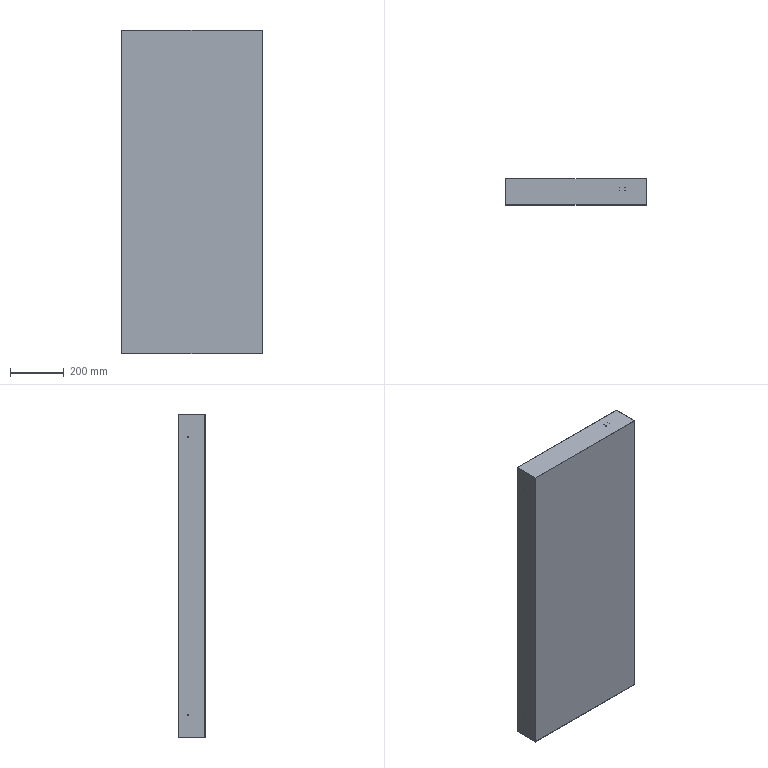Part | SolidWorks | features BaseBody 1 | 1 solid | 27 faces | box 521.763 x 96.993 x 1200 mm | volume 956249 mm3 | cylinder 16 | plane 11 | commonest cylinder face diameters 1.828 x8 3 x8
STEP:
#1=CARTESIAN_POINT('',(-260.881,-535.859,518.28));
#2=VERTEX_POINT('',#1);
#3=CARTESIAN_POINT('',(-260.881,-535.859,515.28));
#4=VERTEX_POINT('',#3);
#5=CARTESIAN_POINT('',(-260.881,-535.859,516.78));
#6=DIRECTION('',(1.,0.,0.));
#7=DIRECTION('',(0.,0.,-1.));
#8=AXIS2_PLACEMENT_3D('',#5,#6,#7);
#9=CIRCLE('',#8,1.5);
#10=EDGE_CURVE('',#2,#4,#9,.T.);
#11=ORIENTED_EDGE('',*,*,#10,.F.);
#12=CARTESIAN_POINT('',(-259.881,-535.859,518.28));
#13=VERTEX_POINT('',#12);
#14=CARTESIAN_POINT('',(-260.881,-535.859,518.28));
#15=DIRECTION('',(1.,0.,0.));
#16=VECTOR('',#15,1000.);
#17=LINE('',#14,#16);
#18=EDGE_CURVE('',#2,#13,#17,.T.);
#19=ORIENTED_EDGE('',*,*,#18,.T.);
#20=CARTESIAN_POINT('',(-259.881,-535.859,515.28));
#21=VERTEX_POINT('',#20);
#22=CARTESIAN_POINT('',(-259.881,-535.859,516.78));
#23=DIRECTION('',(-1.,0.,0.));
#24=DIRECTION('',(0.,0.,-1.));
#25=AXIS2_PLACEMENT_3D('',#22,#23,#24);
#26=CIRCLE('',#25,1.5);
#27=EDGE_CURVE('',#21,#13,#26,.T.);
#28=ORIENTED_EDGE('',*,*,#27,.F.);
#29=CARTESIAN_POINT('',(-260.881,-535.859,515.28));
#30=DIRECTION('',(1.,0.,0.));
#31=VECTOR('',#30,1000.);
#32=LINE('',#29,#31);
#33=EDGE_CURVE('',#4,#21,#32,.T.);
#34=ORIENTED_EDGE('',*,*,#33,.F.);
#35=EDGE_LOOP('',(#11,#19,#28,#34));
#36=FACE_OUTER_BOUND('',#35,.T.);
#37=CARTESIAN_POINT('',(-260.881,-535.859,516.78));
#38=DIRECTION('',(1.,0.,0.));
#39=DIRECTION('',(0.,0.,-1.));
#40=AXIS2_PLACEMENT_3D('',#37,#38,#39);
#41=CYLINDRICAL_SURFACE('',#40,1.5);
#42=ADVANCED_FACE('',(#36),#41,.F.);
#43=CARTESIAN_POINT('',(-260.881,-535.859,-515.72));
#44=VERTEX_POINT('',#43);
#45=CARTESIAN_POINT('',(-260.881,-535.859,-518.72));
#46=VERTEX_POINT('',#45);
#47=CARTESIAN_POINT('',(-260.881,-535.859,-517.22));
#48=DIRECTION('',(1.,0.,0.));
#49=DIRECTION('',(0.,0.,-1.));
#50=AXIS2_PLACEMENT_3D('',#47,#48,#49);
#51=CIRCLE('',#50,1.5);
#52=EDGE_CURVE('',#44,#46,#51,.T.);
#53=ORIENTED_EDGE('',*,*,#52,.F.);
#54=CARTESIAN_POINT('',(-259.881,-535.859,-515.72));
#55=VERTEX_POINT('',#54);
#56=CARTESIAN_POINT('',(-260.881,-535.859,-515.72));
#57=DIRECTION('',(1.,0.,0.));
#58=VECTOR('',#57,1000.);
#59=LINE('',#56,#58);
#60=EDGE_CURVE('',#44,#55,#59,.T.);
#61=ORIENTED_EDGE('',*,*,#60,.T.);
#62=CARTESIAN_POINT('',(-259.881,-535.859,-518.72));
#63=VERTEX_POINT('',#62);
#64=CARTESIAN_POINT('',(-259.881,-535.859,-517.22));
#65=DIRECTION('',(-1.,0.,0.));
#66=DIRECTION('',(0.,0.,-1.));
#67=AXIS2_PLACEMENT_3D('',#64,#65,#66);
#68=CIRCLE('',#67,1.5);
#69=EDGE_CURVE('',#63,#55,#68,.T.);
#70=ORIENTED_EDGE('',*,*,#69,.F.);
#71=CARTESIAN_POINT('',(-260.881,-535.859,-518.72));
#72=DIRECTION('',(1.,0.,0.));
#73=VECTOR('',#72,1000.);
#74=LINE('',#71,#73);
#75=EDGE_CURVE('',#46,#63,#74,.T.);
#76=ORIENTED_EDGE('',*,*,#75,.F.);
#77=EDGE_LOOP('',(#53,#61,#70,#76));
#78=FACE_OUTER_BOUND('',#77,.T.);
#79=CARTESIAN_POINT('',(-260.881,-535.859,-517.22));
#80=DIRECTION('',(1.,0.,0.));
#81=DIRECTION('',(0.,0.,-1.));
#82=AXIS2_PLACEMENT_3D('',#79,#80,#81);
#83=CYLINDRICAL_SURFACE('',#82,1.5);
#84=ADVANCED_FACE('',(#78),#83,.F.);
#85=CARTESIAN_POINT('',(182.261,-534.957,600.));
#86=VERTEX_POINT('',#85);
#87=CARTESIAN_POINT('',(180.433,-534.957,600.));
#88=VERTEX_POINT('',#87);
#89=CARTESIAN_POINT('',(181.347,-534.957,600.));
#90=DIRECTION('',(0.,0.,-1.));
#91=DIRECTION('',(-1.,0.,0.));
#92=AXIS2_PLACEMENT_3D('',#89,#90,#91);
#93=CIRCLE('',#92,0.9139);
#94=EDGE_CURVE('',#86,#88,#93,.T.);
#95=ORIENTED_EDGE('',*,*,#94,.F.);
#96=CARTESIAN_POINT('',(182.261,-534.957,599.));
#97=VERTEX_POINT('',#96);
#98=CARTESIAN_POINT('',(182.261,-534.957,600.));
#99=DIRECTION('',(0.,0.,-1.));
#100=VECTOR('',#99,1000.);
#101=LINE('',#98,#100);
#102=EDGE_CURVE('',#86,#97,#101,.T.);
#103=ORIENTED_EDGE('',*,*,#102,.T.);
#104=CARTESIAN_POINT('',(180.433,-534.957,599.));
#105=VERTEX_POINT('',#104);
#106=CARTESIAN_POINT('',(181.347,-534.957,599.));
#107=DIRECTION('',(0.,0.,1.));
#108=DIRECTION('',(-1.,0.,0.));
#109=AXIS2_PLACEMENT_3D('',#106,#107,#108);
#110=CIRCLE('',#109,0.9139);
#111=EDGE_CURVE('',#105,#97,#110,.T.);
#112=ORIENTED_EDGE('',*,*,#111,.F.);
#113=CARTESIAN_POINT('',(180.433,-534.957,600.));
#114=DIRECTION('',(0.,0.,-1.));
#115=VECTOR('',#114,1000.);
#116=LINE('',#113,#115);
#117=EDGE_CURVE('',#88,#105,#116,.T.);
#118=ORIENTED_EDGE('',*,*,#117,.F.);
#119=EDGE_LOOP('',(#95,#103,#112,#118));
#120=FACE_OUTER_BOUND('',#119,.T.);
#121=CARTESIAN_POINT('',(181.347,-534.957,600.));
#122=DIRECTION('',(0.,0.,-1.));
#123=DIRECTION('',(-1.,0.,0.));
#124=AXIS2_PLACEMENT_3D('',#121,#122,#123);
#125=CYLINDRICAL_SURFACE('',#124,0.9139);
#126=ADVANCED_FACE('',(#120),#125,.F.);
#127=CARTESIAN_POINT('',(162.572,-534.957,600.));
#128=VERTEX_POINT('',#127);
#129=CARTESIAN_POINT('',(160.745,-534.957,600.));
#130=VERTEX_POINT('',#129);
#131=CARTESIAN_POINT('',(161.659,-534.957,600.));
#132=DIRECTION('',(0.,0.,-1.));
#133=DIRECTION('',(-1.,0.,0.));
#134=AXIS2_PLACEMENT_3D('',#131,#132,#133);
#135=CIRCLE('',#134,0.9139);
#136=EDGE_CURVE('',#128,#130,#135,.T.);
#137=ORIENTED_EDGE('',*,*,#136,.F.);
#138=CARTESIAN_POINT('',(162.572,-534.957,599.));
#139=VERTEX_POINT('',#138);
#140=CARTESIAN_POINT('',(162.572,-534.957,600.));
#141=DIRECTION('',(0.,0.,-1.));
#142=VECTOR('',#141,1000.);
#143=LINE('',#140,#142);
#144=EDGE_CURVE('',#128,#139,#143,.T.);
#145=ORIENTED_EDGE('',*,*,#144,.T.);
#146=CARTESIAN_POINT('',(160.745,-534.957,599.));
#147=VERTEX_POINT('',#146);
#148=CARTESIAN_POINT('',(161.659,-534.957,599.));
#149=DIRECTION('',(0.,0.,1.));
#150=DIRECTION('',(-1.,0.,0.));
#151=AXIS2_PLACEMENT_3D('',#148,#149,#150);
#152=CIRCLE('',#151,0.9139);
#153=EDGE_CURVE('',#147,#139,#152,.T.);
#154=ORIENTED_EDGE('',*,*,#153,.F.);
#155=CARTESIAN_POINT('',(160.745,-534.957,600.));
#156=DIRECTION('',(0.,0.,-1.));
#157=VECTOR('',#156,1000.);
#158=LINE('',#155,#157);
#159=EDGE_CURVE('',#130,#147,#158,.T.);
#160=ORIENTED_EDGE('',*,*,#159,.F.);
#161=EDGE_LOOP('',(#137,#145,#154,#160));
#162=FACE_OUTER_BOUND('',#161,.T.);
#163=CARTESIAN_POINT('',(161.659,-534.957,600.));
#164=DIRECTION('',(0.,0.,-1.));
#165=DIRECTION('',(-1.,0.,0.));
#166=AXIS2_PLACEMENT_3D('',#163,#164,#165);
#167=CYLINDRICAL_SURFACE('',#166,0.9139);
#168=ADVANCED_FACE('',(#162),#167,.F.);
#169=CARTESIAN_POINT('',(162.572,-545.874,600.));
#170=VERTEX_POINT('',#169);
#171=CARTESIAN_POINT('',(160.745,-545.874,600.));
#172=VERTEX_POINT('',#171);
#173=CARTESIAN_POINT('',(161.659,-545.874,600.));
#174=DIRECTION('',(0.,0.,-1.));
#175=DIRECTION('',(-1.,0.,0.));
#176=AXIS2_PLACEMENT_3D('',#173,#174,#175);
#177=CIRCLE('',#176,0.9139);
#178=EDGE_CURVE('',#170,#172,#177,.T.);
#179=ORIENTED_EDGE('',*,*,#178,.F.);
#180=CARTESIAN_POINT('',(162.572,-545.874,599.));
#181=VERTEX_POINT('',#180);
#182=CARTESIAN_POINT('',(162.572,-545.874,600.));
#183=DIRECTION('',(0.,0.,-1.));
#184=VECTOR('',#183,1000.);
#185=LINE('',#182,#184);
#186=EDGE_CURVE('',#170,#181,#185,.T.);
#187=ORIENTED_EDGE('',*,*,#186,.T.);
#188=CARTESIAN_POINT('',(160.745,-545.874,599.));
#189=VERTEX_POINT('',#188);
#190=CARTESIAN_POINT('',(161.659,-545.874,599.));
#191=DIRECTION('',(0.,0.,1.));
#192=DIRECTION('',(-1.,0.,0.));
#193=AXIS2_PLACEMENT_3D('',#190,#191,#192);
#194=CIRCLE('',#193,0.9139);
#195=EDGE_CURVE('',#189,#181,#194,.T.);
#196=ORIENTED_EDGE('',*,*,#195,.F.);
#197=CARTESIAN_POINT('',(160.745,-545.874,600.));
#198=DIRECTION('',(0.,0.,-1.));
#199=VECTOR('',#198,1000.);
#200=LINE('',#197,#199);
#201=EDGE_CURVE('',#172,#189,#200,.T.);
#202=ORIENTED_EDGE('',*,*,#201,.F.);
#203=EDGE_LOOP('',(#179,#187,#196,#202));
#204=FACE_OUTER_BOUND('',#203,.T.);
#205=CARTESIAN_POINT('',(161.659,-545.874,600.));
#206=DIRECTION('',(0.,0.,-1.));
#207=DIRECTION('',(-1.,0.,0.));
#208=AXIS2_PLACEMENT_3D('',#205,#206,#207);
#209=CYLINDRICAL_SURFACE('',#208,0.9139);
#210=ADVANCED_FACE('',(#204),#209,.F.);
#211=CARTESIAN_POINT('',(182.261,-545.874,600.));
#212=VERTEX_POINT('',#211);
#213=CARTESIAN_POINT('',(180.433,-545.874,600.));
#214=VERTEX_POINT('',#213);
#215=CARTESIAN_POINT('',(181.347,-545.874,600.));
#216=DIRECTION('',(0.,0.,-1.));
#217=DIRECTION('',(-1.,0.,0.));
#218=AXIS2_PLACEMENT_3D('',#215,#216,#217);
#219=CIRCLE('',#218,0.9139);
#220=EDGE_CURVE('',#212,#214,#219,.T.);
#221=ORIENTED_EDGE('',*,*,#220,.F.);
#222=CARTESIAN_POINT('',(182.261,-545.874,599.));
#223=VERTEX_POINT('',#222);
#224=CARTESIAN_POINT('',(182.261,-545.874,600.));
#225=DIRECTION('',(0.,0.,-1.));
#226=VECTOR('',#225,1000.);
#227=LINE('',#224,#226);
#228=EDGE_CURVE('',#212,#223,#227,.T.);
#229=ORIENTED_EDGE('',*,*,#228,.T.);
#230=CARTESIAN_POINT('',(180.433,-545.874,599.));
#231=VERTEX_POINT('',#230);
#232=CARTESIAN_POINT('',(181.347,-545.874,599.));
#233=DIRECTION('',(0.,0.,1.));
#234=DIRECTION('',(-1.,0.,0.));
#235=AXIS2_PLACEMENT_3D('',#232,#233,#234);
#236=CIRCLE('',#235,0.9139);
#237=EDGE_CURVE('',#231,#223,#236,.T.);
#238=ORIENTED_EDGE('',*,*,#237,.F.);
#239=CARTESIAN_POINT('',(180.433,-545.874,600.));
#240=DIRECTION('',(0.,0.,-1.));
#241=VECTOR('',#240,1000.);
#242=LINE('',#239,#241);
#243=EDGE_CURVE('',#214,#231,#242,.T.);
#244=ORIENTED_EDGE('',*,*,#243,.F.);
#245=EDGE_LOOP('',(#221,#229,#238,#244));
#246=FACE_OUTER_BOUND('',#245,.T.);
#247=CARTESIAN_POINT('',(181.347,-545.874,600.));
#248=DIRECTION('',(0.,0.,-1.));
#249=DIRECTION('',(-1.,0.,0.));
#250=AXIS2_PLACEMENT_3D('',#247,#248,#249);
#251=CYLINDRICAL_SURFACE('',#250,0.9139);
#252=ADVANCED_FACE('',(#246),#251,.F.);
#253=CARTESIAN_POINT('',(259.881,-535.859,518.28));
#254=VERTEX_POINT('',#253);
#255=CARTESIAN_POINT('',(259.881,-535.859,515.28));
#256=VERTEX_POINT('',#255);
#257=CARTESIAN_POINT('',(259.881,-535.859,516.78));
#258=DIRECTION('',(1.,0.,0.));
#259=DIRECTION('',(0.,0.,-1.));
#260=AXIS2_PLACEMENT_3D('',#257,#258,#259);
#261=CIRCLE('',#260,1.5);
#262=EDGE_CURVE('',#254,#256,#261,.T.);
#263=ORIENTED_EDGE('',*,*,#262,.F.);
#264=CARTESIAN_POINT('',(260.881,-535.859,518.28));
#265=VERTEX_POINT('',#264);
#266=CARTESIAN_POINT('',(-260.881,-535.859,518.28));
#267=DIRECTION('',(1.,0.,0.));
#268=VECTOR('',#267,1000.);
#269=LINE('',#266,#268);
#270=EDGE_CURVE('',#254,#265,#269,.T.);
#271=ORIENTED_EDGE('',*,*,#270,.T.);
#272=CARTESIAN_POINT('',(260.881,-535.859,515.28));
#273=VERTEX_POINT('',#272);
#274=CARTESIAN_POINT('',(260.881,-535.859,516.78));
#275=DIRECTION('',(-1.,0.,0.));
#276=DIRECTION('',(0.,0.,-1.));
#277=AXIS2_PLACEMENT_3D('',#274,#275,#276);
#278=CIRCLE('',#277,1.5);
#279=EDGE_CURVE('',#273,#265,#278,.T.);
#280=ORIENTED_EDGE('',*,*,#279,.F.);
#281=CARTESIAN_POINT('',(-260.881,-535.859,515.28));
#282=DIRECTION('',(1.,0.,0.));
#283=VECTOR('',#282,1000.);
#284=LINE('',#281,#283);
#285=EDGE_CURVE('',#256,#273,#284,.T.);
#286=ORIENTED_EDGE('',*,*,#285,.F.);
#287=EDGE_LOOP('',(#263,#271,#280,#286));
#288=FACE_OUTER_BOUND('',#287,.T.);
#289=CARTESIAN_POINT('',(-260.881,-535.859,516.78));
#290=DIRECTION('',(1.,0.,0.));
#291=DIRECTION('',(0.,0.,-1.));
#292=AXIS2_PLACEMENT_3D('',#289,#290,#291);
#293=CYLINDRICAL_SURFACE('',#292,1.5);
#294=ADVANCED_FACE('',(#288),#293,.F.);
#295=CARTESIAN_POINT('',(259.881,-535.859,-515.72));
#296=VERTEX_POINT('',#295);
#297=CARTESIAN_POINT('',(259.881,-535.859,-518.72));
#298=VERTEX_POINT('',#297);
#299=CARTESIAN_POINT('',(259.881,-535.859,-517.22));
#300=DIRECTION('',(1.,0.,0.));
#301=DIRECTION('',(0.,0.,-1.));
#302=AXIS2_PLACEMENT_3D('',#299,#300,#301);
#303=CIRCLE('',#302,1.5);
#304=EDGE_CURVE('',#296,#298,#303,.T.);
#305=ORIENTED_EDGE('',*,*,#304,.F.);
#306=CARTESIAN_POINT('',(260.881,-535.859,-515.72));
#307=VERTEX_POINT('',#306);
#308=CARTESIAN_POINT('',(-260.881,-535.859,-515.72));
#309=DIRECTION('',(1.,0.,0.));
#310=VECTOR('',#309,1000.);
#311=LINE('',#308,#310);
#312=EDGE_CURVE('',#296,#307,#311,.T.);
#313=ORIENTED_EDGE('',*,*,#312,.T.);
#314=CARTESIAN_POINT('',(260.881,-535.859,-518.72));
#315=VERTEX_POINT('',#314);
#316=CARTESIAN_POINT('',(260.881,-535.859,-517.22));
#317=DIRECTION('',(-1.,0.,0.));
#318=DIRECTION('',(0.,0.,-1.));
#319=AXIS2_PLACEMENT_3D('',#316,#317,#318);
#320=CIRCLE('',#319,1.5);
#321=EDGE_CURVE('',#315,#307,#320,.T.);
#322=ORIENTED_EDGE('',*,*,#321,.F.);
#323=CARTESIAN_POINT('',(-260.881,-535.859,-518.72));
#324=DIRECTION('',(1.,0.,0.));
#325=VECTOR('',#324,1000.);
#326=LINE('',#323,#325);
#327=EDGE_CURVE('',#298,#315,#326,.T.);
#328=ORIENTED_EDGE('',*,*,#327,.F.);
#329=EDGE_LOOP('',(#305,#313,#322,#328));
#330=FACE_OUTER_BOUND('',#329,.T.);
#331=CARTESIAN_POINT('',(-260.881,-535.859,-517.22));
#332=DIRECTION('',(1.,0.,0.));
#333=DIRECTION('',(0.,0.,-1.));
#334=AXIS2_PLACEMENT_3D('',#331,#332,#333);
#335=CYLINDRICAL_SURFACE('',#334,1.5);
#336=ADVANCED_FACE('',(#330),#335,.F.);
#337=CARTESIAN_POINT('',(-260.881,-598.676,600.));
#338=VERTEX_POINT('',#337);
#339=CARTESIAN_POINT('',(-260.881,-598.676,-600.));
#340=VERTEX_POINT('',#339);
#341=CARTESIAN_POINT('',(-260.881,-598.676,0.));
#342=DIRECTION('',(0.,0.,-1.));
#343=VECTOR('',#342,1000.);
#344=LINE('',#341,#343);
#345=EDGE_CURVE('',#338,#340,#344,.T.);
#346=ORIENTED_EDGE('',*,*,#345,.T.);
#347=CARTESIAN_POINT('',(260.881,-598.676,-600.));
#348=VERTEX_POINT('',#347);
#349=CARTESIAN_POINT('',(-260.881,-598.676,-600.));
#350=DIRECTION('',(1.,0.,0.));
#351=VECTOR('',#350,1000.);
#352=LINE('',#349,#351);
#353=EDGE_CURVE('',#340,#348,#352,.T.);
#354=ORIENTED_EDGE('',*,*,#353,.T.);
#355=CARTESIAN_POINT('',(260.881,-598.676,600.));
#356=VERTEX_POINT('',#355);
#357=CARTESIAN_POINT('',(260.881,-598.676,0.));
#358=DIRECTION('',(0.,0.,1.));
#359=VECTOR('',#358,1000.);
#360=LINE('',#357,#359);
#361=EDGE_CURVE('',#348,#356,#360,.T.);
#362=ORIENTED_EDGE('',*,*,#361,.T.);
#363=CARTESIAN_POINT('',(-260.881,-598.676,600.));
#364=DIRECTION('',(-1.,0.,0.));
#365=VECTOR('',#364,1000.);
#366=LINE('',#363,#365);
#367=EDGE_CURVE('',#356,#338,#366,.T.);
#368=ORIENTED_EDGE('',*,*,#367,.T.);
#369=EDGE_LOOP('',(#346,#354,#362,#368));
#370=FACE_OUTER_BOUND('',#369,.T.);
#371=CARTESIAN_POINT('',(-260.881,-598.676,0.));
#372=DIRECTION('',(0.,-1.,0.));
#373=DIRECTION('',(0.,0.,-1.));
#374=AXIS2_PLACEMENT_3D('',#371,#372,#373);
#375=PLANE('',#374);
#376=ADVANCED_FACE('',(#370),#375,.T.);
#377=CARTESIAN_POINT('',(-260.881,-501.682,-600.));
#378=VERTEX_POINT('',#377);
#379=CARTESIAN_POINT('',(260.881,-501.682,-600.));
#380=VERTEX_POINT('',#379);
#381=CARTESIAN_POINT('',(0.,-501.682,-600.));
#382=DIRECTION('',(1.,0.,0.));
#383=VECTOR('',#382,1000.);
#384=LINE('',#381,#383);
#385=EDGE_CURVE('',#378,#380,#384,.T.);
#386=ORIENTED_EDGE('',*,*,#385,.T.);
#387=CARTESIAN_POINT('',(260.881,-550.179,-600.));
#388=DIRECTION('',(0.,-1.,0.));
#389=VECTOR('',#388,1000.);
#390=LINE('',#387,#389);
#391=EDGE_CURVE('',#380,#348,#390,.T.);
#392=ORIENTED_EDGE('',*,*,#391,.T.);
#393=ORIENTED_EDGE('',*,*,#353,.F.);
#394=CARTESIAN_POINT('',(-260.881,-550.179,-600.));
#395=DIRECTION('',(0.,1.,0.));
#396=VECTOR('',#395,1000.);
#397=LINE('',#394,#396);
#398=EDGE_CURVE('',#340,#378,#397,.T.);
#399=ORIENTED_EDGE('',*,*,#398,.T.);
#400=EDGE_LOOP('',(#386,#392,#393,#399));
#401=FACE_OUTER_BOUND('',#400,.T.);
#402=CARTESIAN_POINT('',(0.,-550.179,-600.));
#403=DIRECTION('',(0.,0.,-1.));
#404=DIRECTION('',(-1.,0.,0.));
#405=AXIS2_PLACEMENT_3D('',#402,#403,#404);
#406=PLANE('',#405);
#407=ADVANCED_FACE('',(#401),#406,.T.);
#408=CARTESIAN_POINT('',(-260.881,-535.859,516.78));
#409=DIRECTION('',(1.,0.,0.));
#410=DIRECTION('',(0.,0.,-1.));
#411=AXIS2_PLACEMENT_3D('',#408,#409,#410);
#412=CIRCLE('',#411,1.5);
#413=EDGE_CURVE('',#4,#2,#412,.T.);
#414=ORIENTED_EDGE('',*,*,#413,.T.);
#415=ORIENTED_EDGE('',*,*,#10,.T.);
#416=EDGE_LOOP('',(#414,#415));
#417=FACE_BOUND('',#416,.T.);
#418=CARTESIAN_POINT('',(-260.881,-535.859,-517.22));
#419=DIRECTION('',(1.,0.,0.));
#420=DIRECTION('',(0.,0.,-1.));
#421=AXIS2_PLACEMENT_3D('',#418,#419,#420);
#422=CIRCLE('',#421,1.5);
#423=EDGE_CURVE('',#46,#44,#422,.T.);
#424=ORIENTED_EDGE('',*,*,#423,.T.);
#425=ORIENTED_EDGE('',*,*,#52,.T.);
#426=EDGE_LOOP('',(#424,#425));
#427=FACE_BOUND('',#426,.T.);
#428=CARTESIAN_POINT('',(-260.881,-501.682,600.));
#429=VERTEX_POINT('',#428);
#430=CARTESIAN_POINT('',(-260.881,-501.682,0.));
#431=DIRECTION('',(0.,0.,-1.));
#432=VECTOR('',#431,1000.);
#433=LINE('',#430,#432);
#434=EDGE_CURVE('',#429,#378,#433,.T.);
#435=ORIENTED_EDGE('',*,*,#434,.T.);
#436=ORIENTED_EDGE('',*,*,#398,.F.);
#437=ORIENTED_EDGE('',*,*,#345,.F.);
#438=CARTESIAN_POINT('',(-260.881,-501.682,600.));
#439=DIRECTION('',(0.,1.,0.));
#440=VECTOR('',#439,1000.);
#441=LINE('',#438,#440);
#442=EDGE_CURVE('',#338,#429,#441,.T.);
#443=ORIENTED_EDGE('',*,*,#442,.T.);
#444=EDGE_LOOP('',(#435,#436,#437,#443));
#445=FACE_OUTER_BOUND('',#444,.T.);
#446=CARTESIAN_POINT('',(-260.881,-501.682,0.));
#447=DIRECTION('',(-1.,0.,0.));
#448=DIRECTION('',(0.,0.,1.));
#449=AXIS2_PLACEMENT_3D('',#446,#447,#448);
#450=PLANE('',#449);
#451=ADVANCED_FACE('',(#417,#427,#445),#450,.T.);
#452=CARTESIAN_POINT('',(181.347,-534.957,600.));
#453=DIRECTION('',(0.,0.,-1.));
#454=DIRECTION('',(-1.,0.,0.));
#455=AXIS2_PLACEMENT_3D('',#452,#453,#454);
#456=CIRCLE('',#455,0.9139);
#457=EDGE_CURVE('',#88,#86,#456,.T.);
#458=ORIENTED_EDGE('',*,*,#457,.T.);
#459=ORIENTED_EDGE('',*,*,#94,.T.);
#460=EDGE_LOOP('',(#458,#459));
#461=FACE_BOUND('',#460,.T.);
#462=CARTESIAN_POINT('',(161.659,-534.957,600.));
#463=DIRECTION('',(0.,0.,-1.));
#464=DIRECTION('',(-1.,0.,0.));
#465=AXIS2_PLACEMENT_3D('',#462,#463,#464);
#466=CIRCLE('',#465,0.9139);
#467=EDGE_CURVE('',#130,#128,#466,.T.);
#468=ORIENTED_EDGE('',*,*,#467,.T.);
#469=ORIENTED_EDGE('',*,*,#136,.T.);
#470=EDGE_LOOP('',(#468,#469));
#471=FACE_BOUND('',#470,.T.);
#472=CARTESIAN_POINT('',(161.659,-545.874,600.));
#473=DIRECTION('',(0.,0.,-1.));
#474=DIRECTION('',(-1.,0.,0.));
#475=AXIS2_PLACEMENT_3D('',#472,#473,#474);
#476=CIRCLE('',#475,0.9139);
#477=EDGE_CURVE('',#172,#170,#476,.T.);
#478=ORIENTED_EDGE('',*,*,#477,.T.);
#479=ORIENTED_EDGE('',*,*,#178,.T.);
#480=EDGE_LOOP('',(#478,#479));
#481=FACE_BOUND('',#480,.T.);
#482=CARTESIAN_POINT('',(181.347,-545.874,600.));
#483=DIRECTION('',(0.,0.,-1.));
#484=DIRECTION('',(-1.,0.,0.));
#485=AXIS2_PLACEMENT_3D('',#482,#483,#484);
#486=CIRCLE('',#485,0.9139);
#487=EDGE_CURVE('',#214,#212,#486,.T.);
#488=ORIENTED_EDGE('',*,*,#487,.T.);
#489=ORIENTED_EDGE('',*,*,#220,.T.);
#490=EDGE_LOOP('',(#488,#489));
#491=FACE_BOUND('',#490,.T.);
#492=CARTESIAN_POINT('',(260.881,-501.682,600.));
#493=VERTEX_POINT('',#492);
#494=CARTESIAN_POINT('',(0.,-501.682,600.));
#495=DIRECTION('',(-1.,0.,0.));
#496=VECTOR('',#495,1000.);
#497=LINE('',#494,#496);
#498=EDGE_CURVE('',#493,#429,#497,.T.);
#499=ORIENTED_EDGE('',*,*,#498,.T.);
#500=ORIENTED_EDGE('',*,*,#442,.F.);
#501=ORIENTED_EDGE('',*,*,#367,.F.);
#502=CARTESIAN_POINT('',(260.881,-550.179,600.));
#503=DIRECTION('',(0.,1.,0.));
#504=VECTOR('',#503,1000.);
#505=LINE('',#502,#504);
#506=EDGE_CURVE('',#356,#493,#505,.T.);
#507=ORIENTED_EDGE('',*,*,#506,.T.);
#508=EDGE_LOOP('',(#499,#500,#501,#507));
#509=FACE_OUTER_BOUND('',#508,.T.);
#510=CARTESIAN_POINT('',(0.,-550.179,600.));
#511=DIRECTION('',(0.,0.,1.));
#512=DIRECTION('',(1.,0.,0.));
#513=AXIS2_PLACEMENT_3D('',#510,#511,#512);
#514=PLANE('',#513);
#515=ADVANCED_FACE('',(#461,#471,#481,#491,#509),#514,.T.);
#516=ORIENTED_EDGE('',*,*,#279,.T.);
#517=CARTESIAN_POINT('',(260.881,-535.859,516.78));
#518=DIRECTION('',(-1.,0.,0.));
#519=DIRECTION('',(0.,0.,-1.));
#520=AXIS2_PLACEMENT_3D('',#517,#518,#519);
#521=CIRCLE('',#520,1.5);
#522=EDGE_CURVE('',#265,#273,#521,.T.);
#523=ORIENTED_EDGE('',*,*,#522,.T.);
#524=EDGE_LOOP('',(#516,#523));
#525=FACE_BOUND('',#524,.T.);
#526=ORIENTED_EDGE('',*,*,#321,.T.);
#527=CARTESIAN_POINT('',(260.881,-535.859,-517.22));
#528=DIRECTION('',(-1.,0.,0.));
#529=DIRECTION('',(0.,0.,-1.));
#530=AXIS2_PLACEMENT_3D('',#527,#528,#529);
#531=CIRCLE('',#530,1.5);
#532=EDGE_CURVE('',#307,#315,#531,.T.);
#533=ORIENTED_EDGE('',*,*,#532,.T.);
#534=EDGE_LOOP('',(#526,#533));
#535=FACE_BOUND('',#534,.T.);
#536=ORIENTED_EDGE('',*,*,#361,.F.);
#537=ORIENTED_EDGE('',*,*,#391,.F.);
#538=CARTESIAN_POINT('',(260.881,-501.682,0.));
#539=DIRECTION('',(0.,0.,1.));
#540=VECTOR('',#539,1000.);
#541=LINE('',#538,#540);
#542=EDGE_CURVE('',#380,#493,#541,.T.);
#543=ORIENTED_EDGE('',*,*,#542,.T.);
#544=ORIENTED_EDGE('',*,*,#506,.F.);
#545=EDGE_LOOP('',(#536,#537,#543,#544));
#546=FACE_OUTER_BOUND('',#545,.T.);
#547=CARTESIAN_POINT('',(260.881,-598.676,0.));
#548=DIRECTION('',(1.,0.,0.));
#549=DIRECTION('',(0.,0.,-1.));
#550=AXIS2_PLACEMENT_3D('',#547,#548,#549);
#551=PLANE('',#550);
#552=ADVANCED_FACE('',(#525,#535,#546),#551,.T.);
#553=CARTESIAN_POINT('',(259.881,-501.682,599.));
#554=VERTEX_POINT('',#553);
#555=CARTESIAN_POINT('',(-259.881,-501.682,599.));
#556=VERTEX_POINT('',#555);
#557=CARTESIAN_POINT('',(260.881,-501.682,599.));
#558=DIRECTION('',(-1.,0.,0.));
#559=VECTOR('',#558,1000.);
#560=LINE('',#557,#559);
#561=EDGE_CURVE('',#554,#556,#560,.T.);
#562=ORIENTED_EDGE('',*,*,#561,.T.);
#563=CARTESIAN_POINT('',(-259.881,-501.682,-599.));
#564=VERTEX_POINT('',#563);
#565=CARTESIAN_POINT('',(-259.881,-501.682,0.));
#566=DIRECTION('',(0.,0.,-1.));
#567=VECTOR('',#566,1000.);
#568=LINE('',#565,#567);
#569=EDGE_CURVE('',#556,#564,#568,.T.);
#570=ORIENTED_EDGE('',*,*,#569,.T.);
#571=CARTESIAN_POINT('',(259.881,-501.682,-599.));
#572=VERTEX_POINT('',#571);
#573=CARTESIAN_POINT('',(260.881,-501.682,-599.));
#574=DIRECTION('',(1.,0.,0.));
#575=VECTOR('',#574,1000.);
#576=LINE('',#573,#575);
#577=EDGE_CURVE('',#564,#572,#576,.T.);
#578=ORIENTED_EDGE('',*,*,#577,.T.);
#579=CARTESIAN_POINT('',(259.881,-501.682,0.));
#580=DIRECTION('',(0.,0.,1.));
#581=VECTOR('',#580,1000.);
#582=LINE('',#579,#581);
#583=EDGE_CURVE('',#572,#554,#582,.T.);
#584=ORIENTED_EDGE('',*,*,#583,.T.);
#585=EDGE_LOOP('',(#562,#570,#578,#584));
#586=FACE_BOUND('',#585,.T.);
#587=ORIENTED_EDGE('',*,*,#542,.F.);
#588=ORIENTED_EDGE('',*,*,#385,.F.);
#589=ORIENTED_EDGE('',*,*,#434,.F.);
#590=ORIENTED_EDGE('',*,*,#498,.F.);
#591=EDGE_LOOP('',(#587,#588,#589,#590));
#592=FACE_OUTER_BOUND('',#591,.T.);
#593=CARTESIAN_POINT('',(260.881,-501.682,0.));
#594=DIRECTION('',(0.,1.,0.));
#595=DIRECTION('',(0.,0.,1.));
#596=AXIS2_PLACEMENT_3D('',#593,#594,#595);
#597=PLANE('',#596);
#598=ADVANCED_FACE('',(#586,#592),#597,.T.);
#599=ORIENTED_EDGE('',*,*,#18,.F.);
#600=ORIENTED_EDGE('',*,*,#413,.F.);
#601=ORIENTED_EDGE('',*,*,#33,.T.);
#602=CARTESIAN_POINT('',(-259.881,-535.859,516.78));
#603=DIRECTION('',(-1.,0.,0.));
#604=DIRECTION('',(0.,0.,-1.));
#605=AXIS2_PLACEMENT_3D('',#602,#603,#604);
#606=CIRCLE('',#605,1.5);
#607=EDGE_CURVE('',#13,#21,#606,.T.);
#608=ORIENTED_EDGE('',*,*,#607,.F.);
#609=EDGE_LOOP('',(#599,#600,#601,#608));
#610=FACE_OUTER_BOUND('',#609,.T.);
#611=CARTESIAN_POINT('',(-260.881,-535.859,516.78));
#612=DIRECTION('',(1.,0.,0.));
#613=DIRECTION('',(0.,0.,-1.));
#614=AXIS2_PLACEMENT_3D('',#611,#612,#613);
#615=CYLINDRICAL_SURFACE('',#614,1.5);
#616=ADVANCED_FACE('',(#610),#615,.F.);
#617=ORIENTED_EDGE('',*,*,#60,.F.);
#618=ORIENTED_EDGE('',*,*,#423,.F.);
#619=ORIENTED_EDGE('',*,*,#75,.T.);
#620=CARTESIAN_POINT('',(-259.881,-535.859,-517.22));
#621=DIRECTION('',(-1.,0.,0.));
#622=DIRECTION('',(0.,0.,-1.));
#623=AXIS2_PLACEMENT_3D('',#620,#621,#622);
#624=CIRCLE('',#623,1.5);
#625=EDGE_CURVE('',#55,#63,#624,.T.);
#626=ORIENTED_EDGE('',*,*,#625,.F.);
#627=EDGE_LOOP('',(#617,#618,#619,#626));
#628=FACE_OUTER_BOUND('',#627,.T.);
#629=CARTESIAN_POINT('',(-260.881,-535.859,-517.22));
#630=DIRECTION('',(1.,0.,0.));
#631=DIRECTION('',(0.,0.,-1.));
#632=AXIS2_PLACEMENT_3D('',#629,#630,#631);
#633=CYLINDRICAL_SURFACE('',#632,1.5);
#634=ADVANCED_FACE('',(#628),#633,.F.);
#635=ORIENTED_EDGE('',*,*,#102,.F.);
#636=ORIENTED_EDGE('',*,*,#457,.F.);
#637=ORIENTED_EDGE('',*,*,#117,.T.);
#638=CARTESIAN_POINT('',(181.347,-534.957,599.));
#639=DIRECTION('',(0.,0.,1.));
#640=DIRECTION('',(-1.,0.,0.));
#641=AXIS2_PLACEMENT_3D('',#638,#639,#640);
#642=CIRCLE('',#641,0.9139);
#643=EDGE_CURVE('',#97,#105,#642,.T.);
#644=ORIENTED_EDGE('',*,*,#643,.F.);
#645=EDGE_LOOP('',(#635,#636,#637,#644));
#646=FACE_OUTER_BOUND('',#645,.T.);
#647=CARTESIAN_POINT('',(181.347,-534.957,600.));
#648=DIRECTION('',(0.,0.,-1.));
#649=DIRECTION('',(-1.,0.,0.));
#650=AXIS2_PLACEMENT_3D('',#647,#648,#649);
#651=CYLINDRICAL_SURFACE('',#650,0.9139);
#652=ADVANCED_FACE('',(#646),#651,.F.);
#653=ORIENTED_EDGE('',*,*,#144,.F.);
#654=ORIENTED_EDGE('',*,*,#467,.F.);
#655=ORIENTED_EDGE('',*,*,#159,.T.);
#656=CARTESIAN_POINT('',(161.659,-534.957,599.));
#657=DIRECTION('',(0.,0.,1.));
#658=DIRECTION('',(-1.,0.,0.));
#659=AXIS2_PLACEMENT_3D('',#656,#657,#658);
#660=CIRCLE('',#659,0.9139);
#661=EDGE_CURVE('',#139,#147,#660,.T.);
#662=ORIENTED_EDGE('',*,*,#661,.F.);
#663=EDGE_LOOP('',(#653,#654,#655,#662));
#664=FACE_OUTER_BOUND('',#663,.T.);
#665=CARTESIAN_POINT('',(161.659,-534.957,600.));
#666=DIRECTION('',(0.,0.,-1.));
#667=DIRECTION('',(-1.,0.,0.));
#668=AXIS2_PLACEMENT_3D('',#665,#666,#667);
#669=CYLINDRICAL_SURFACE('',#668,0.9139);
#670=ADVANCED_FACE('',(#664),#669,.F.);
#671=ORIENTED_EDGE('',*,*,#186,.F.);
#672=ORIENTED_EDGE('',*,*,#477,.F.);
#673=ORIENTED_EDGE('',*,*,#201,.T.);
#674=CARTESIAN_POINT('',(161.659,-545.874,599.));
#675=DIRECTION('',(0.,0.,1.));
#676=DIRECTION('',(-1.,0.,0.));
#677=AXIS2_PLACEMENT_3D('',#674,#675,#676);
#678=CIRCLE('',#677,0.9139);
#679=EDGE_CURVE('',#181,#189,#678,.T.);
#680=ORIENTED_EDGE('',*,*,#679,.F.);
#681=EDGE_LOOP('',(#671,#672,#673,#680));
#682=FACE_OUTER_BOUND('',#681,.T.);
#683=CARTESIAN_POINT('',(161.659,-545.874,600.));
#684=DIRECTION('',(0.,0.,-1.));
#685=DIRECTION('',(-1.,0.,0.));
#686=AXIS2_PLACEMENT_3D('',#683,#684,#685);
#687=CYLINDRICAL_SURFACE('',#686,0.9139);
#688=ADVANCED_FACE('',(#682),#687,.F.);
#689=ORIENTED_EDGE('',*,*,#228,.F.);
#690=ORIENTED_EDGE('',*,*,#487,.F.);
#691=ORIENTED_EDGE('',*,*,#243,.T.);
#692=CARTESIAN_POINT('',(181.347,-545.874,599.));
#693=DIRECTION('',(0.,0.,1.));
#694=DIRECTION('',(-1.,0.,0.));
#695=AXIS2_PLACEMENT_3D('',#692,#693,#694);
#696=CIRCLE('',#695,0.9139);
#697=EDGE_CURVE('',#223,#231,#696,.T.);
#698=ORIENTED_EDGE('',*,*,#697,.F.);
#699=EDGE_LOOP('',(#689,#690,#691,#698));
#700=FACE_OUTER_BOUND('',#699,.T.);
#701=CARTESIAN_POINT('',(181.347,-545.874,600.));
#702=DIRECTION('',(0.,0.,-1.));
#703=DIRECTION('',(-1.,0.,0.));
#704=AXIS2_PLACEMENT_3D('',#701,#702,#703);
#705=CYLINDRICAL_SURFACE('',#704,0.9139);
#706=ADVANCED_FACE('',(#700),#705,.F.);
#707=ORIENTED_EDGE('',*,*,#270,.F.);
#708=CARTESIAN_POINT('',(259.881,-535.859,516.78));
#709=DIRECTION('',(1.,0.,0.));
#710=DIRECTION('',(0.,0.,-1.));
#711=AXIS2_PLACEMENT_3D('',#708,#709,#710);
#712=CIRCLE('',#711,1.5);
#713=EDGE_CURVE('',#256,#254,#712,.T.);
#714=ORIENTED_EDGE('',*,*,#713,.F.);
#715=ORIENTED_EDGE('',*,*,#285,.T.);
#716=ORIENTED_EDGE('',*,*,#522,.F.);
#717=EDGE_LOOP('',(#707,#714,#715,#716));
#718=FACE_OUTER_BOUND('',#717,.T.);
#719=CARTESIAN_POINT('',(-260.881,-535.859,516.78));
#720=DIRECTION('',(1.,0.,0.));
#721=DIRECTION('',(0.,0.,-1.));
#722=AXIS2_PLACEMENT_3D('',#719,#720,#721);
#723=CYLINDRICAL_SURFACE('',#722,1.5);
#724=ADVANCED_FACE('',(#718),#723,.F.);
#725=ORIENTED_EDGE('',*,*,#312,.F.);
#726=CARTESIAN_POINT('',(259.881,-535.859,-517.22));
#727=DIRECTION('',(1.,0.,0.));
#728=DIRECTION('',(0.,0.,-1.));
#729=AXIS2_PLACEMENT_3D('',#726,#727,#728);
#730=CIRCLE('',#729,1.5);
#731=EDGE_CURVE('',#298,#296,#730,.T.);
#732=ORIENTED_EDGE('',*,*,#731,.F.);
#733=ORIENTED_EDGE('',*,*,#327,.T.);
#734=ORIENTED_EDGE('',*,*,#532,.F.);
#735=EDGE_LOOP('',(#725,#732,#733,#734));
#736=FACE_OUTER_BOUND('',#735,.T.);
#737=CARTESIAN_POINT('',(-260.881,-535.859,-517.22));
#738=DIRECTION('',(1.,0.,0.));
#739=DIRECTION('',(0.,0.,-1.));
#740=AXIS2_PLACEMENT_3D('',#737,#738,#739);
#741=CYLINDRICAL_SURFACE('',#740,1.5);
#742=ADVANCED_FACE('',(#736),#741,.F.);
#743=ORIENTED_EDGE('',*,*,#27,.T.);
#744=ORIENTED_EDGE('',*,*,#607,.T.);
#745=EDGE_LOOP('',(#743,#744));
#746=FACE_BOUND('',#745,.T.);
#747=ORIENTED_EDGE('',*,*,#69,.T.);
#748=ORIENTED_EDGE('',*,*,#625,.T.);
#749=EDGE_LOOP('',(#747,#748));
#750=FACE_BOUND('',#749,.T.);
#751=CARTESIAN_POINT('',(-259.881,-597.676,-599.));
#752=VERTEX_POINT('',#751);
#753=CARTESIAN_POINT('',(-259.881,-501.682,-599.));
#754=DIRECTION('',(0.,-1.,0.));
#755=VECTOR('',#754,1000.);
#756=LINE('',#753,#755);
#757=EDGE_CURVE('',#564,#752,#756,.T.);
#758=ORIENTED_EDGE('',*,*,#757,.F.);
#759=ORIENTED_EDGE('',*,*,#569,.F.);
#760=CARTESIAN_POINT('',(-259.881,-597.676,599.));
#761=VERTEX_POINT('',#760);
#762=CARTESIAN_POINT('',(-259.881,-501.682,599.));
#763=DIRECTION('',(0.,1.,0.));
#764=VECTOR('',#763,1000.);
#765=LINE('',#762,#764);
#766=EDGE_CURVE('',#761,#556,#765,.T.);
#767=ORIENTED_EDGE('',*,*,#766,.F.);
#768=CARTESIAN_POINT('',(-259.881,-597.676,0.));
#769=DIRECTION('',(0.,0.,1.));
#770=VECTOR('',#769,1000.);
#771=LINE('',#768,#770);
#772=EDGE_CURVE('',#752,#761,#771,.T.);
#773=ORIENTED_EDGE('',*,*,#772,.F.);
#774=EDGE_LOOP('',(#758,#759,#767,#773));
#775=FACE_OUTER_BOUND('',#774,.T.);
#776=CARTESIAN_POINT('',(-259.881,-501.682,0.));
#777=DIRECTION('',(-1.,0.,0.));
#778=DIRECTION('',(0.,0.,1.));
#779=AXIS2_PLACEMENT_3D('',#776,#777,#778);
#780=PLANE('',#779);
#781=ADVANCED_FACE('',(#746,#750,#775),#780,.F.);
#782=ORIENTED_EDGE('',*,*,#111,.T.);
#783=ORIENTED_EDGE('',*,*,#643,.T.);
#784=EDGE_LOOP('',(#782,#783));
#785=FACE_BOUND('',#784,.T.);
#786=ORIENTED_EDGE('',*,*,#153,.T.);
#787=ORIENTED_EDGE('',*,*,#661,.T.);
#788=EDGE_LOOP('',(#786,#787));
#789=FACE_BOUND('',#788,.T.);
#790=ORIENTED_EDGE('',*,*,#195,.T.);
#791=ORIENTED_EDGE('',*,*,#679,.T.);
#792=EDGE_LOOP('',(#790,#791));
#793=FACE_BOUND('',#792,.T.);
#794=ORIENTED_EDGE('',*,*,#237,.T.);
#795=ORIENTED_EDGE('',*,*,#697,.T.);
#796=EDGE_LOOP('',(#794,#795));
#797=FACE_BOUND('',#796,.T.);
#798=ORIENTED_EDGE('',*,*,#766,.T.);
#799=ORIENTED_EDGE('',*,*,#561,.F.);
#800=CARTESIAN_POINT('',(259.881,-597.676,599.));
#801=VERTEX_POINT('',#800);
#802=CARTESIAN_POINT('',(259.881,-550.179,599.));
#803=DIRECTION('',(0.,1.,0.));
#804=VECTOR('',#803,1000.);
#805=LINE('',#802,#804);
#806=EDGE_CURVE('',#801,#554,#805,.T.);
#807=ORIENTED_EDGE('',*,*,#806,.F.);
#808=CARTESIAN_POINT('',(0.,-597.676,599.));
#809=DIRECTION('',(1.,0.,0.));
#810=VECTOR('',#809,1000.);
#811=LINE('',#808,#810);
#812=EDGE_CURVE('',#761,#801,#811,.T.);
#813=ORIENTED_EDGE('',*,*,#812,.F.);
#814=EDGE_LOOP('',(#798,#799,#807,#813));
#815=FACE_OUTER_BOUND('',#814,.T.);
#816=CARTESIAN_POINT('',(0.,-550.179,599.));
#817=DIRECTION('',(0.,0.,1.));
#818=DIRECTION('',(1.,0.,0.));
#819=AXIS2_PLACEMENT_3D('',#816,#817,#818);
#820=PLANE('',#819);
#821=ADVANCED_FACE('',(#785,#789,#793,#797,#815),#820,.F.);
#822=ORIENTED_EDGE('',*,*,#713,.T.);
#823=ORIENTED_EDGE('',*,*,#262,.T.);
#824=EDGE_LOOP('',(#822,#823));
#825=FACE_BOUND('',#824,.T.);
#826=ORIENTED_EDGE('',*,*,#731,.T.);
#827=ORIENTED_EDGE('',*,*,#304,.T.);
#828=EDGE_LOOP('',(#826,#827));
#829=FACE_BOUND('',#828,.T.);
#830=CARTESIAN_POINT('',(259.881,-597.676,-599.));
#831=VERTEX_POINT('',#830);
#832=CARTESIAN_POINT('',(259.881,-598.676,-599.));
#833=DIRECTION('',(0.,1.,0.));
#834=VECTOR('',#833,1000.);
#835=LINE('',#832,#834);
#836=EDGE_CURVE('',#831,#572,#835,.T.);
#837=ORIENTED_EDGE('',*,*,#836,.F.);
#838=CARTESIAN_POINT('',(259.881,-597.676,0.));
#839=DIRECTION('',(0.,0.,-1.));
#840=VECTOR('',#839,1000.);
#841=LINE('',#838,#840);
#842=EDGE_CURVE('',#801,#831,#841,.T.);
#843=ORIENTED_EDGE('',*,*,#842,.F.);
#844=ORIENTED_EDGE('',*,*,#806,.T.);
#845=ORIENTED_EDGE('',*,*,#583,.F.);
#846=EDGE_LOOP('',(#837,#843,#844,#845));
#847=FACE_OUTER_BOUND('',#846,.T.);
#848=CARTESIAN_POINT('',(259.881,-598.676,0.));
#849=DIRECTION('',(1.,0.,0.));
#850=DIRECTION('',(0.,0.,-1.));
#851=AXIS2_PLACEMENT_3D('',#848,#849,#850);
#852=PLANE('',#851);
#853=ADVANCED_FACE('',(#825,#829,#847),#852,.F.);
#854=ORIENTED_EDGE('',*,*,#836,.T.);
#855=ORIENTED_EDGE('',*,*,#577,.F.);
#856=ORIENTED_EDGE('',*,*,#757,.T.);
#857=CARTESIAN_POINT('',(0.,-597.676,-599.));
#858=DIRECTION('',(-1.,0.,0.));
#859=VECTOR('',#858,1000.);
#860=LINE('',#857,#859);
#861=EDGE_CURVE('',#831,#752,#860,.T.);
#862=ORIENTED_EDGE('',*,*,#861,.F.);
#863=EDGE_LOOP('',(#854,#855,#856,#862));
#864=FACE_OUTER_BOUND('',#863,.T.);
#865=CARTESIAN_POINT('',(0.,-550.179,-599.));
#866=DIRECTION('',(0.,0.,-1.));
#867=DIRECTION('',(-1.,0.,0.));
#868=AXIS2_PLACEMENT_3D('',#865,#866,#867);
#869=PLANE('',#868);
#870=ADVANCED_FACE('',(#864),#869,.F.);
#871=ORIENTED_EDGE('',*,*,#861,.T.);
#872=ORIENTED_EDGE('',*,*,#772,.T.);
#873=ORIENTED_EDGE('',*,*,#812,.T.);
#874=ORIENTED_EDGE('',*,*,#842,.T.);
#875=EDGE_LOOP('',(#871,#872,#873,#874));
#876=FACE_OUTER_BOUND('',#875,.T.);
#877=CARTESIAN_POINT('',(-260.881,-597.676,0.));
#878=DIRECTION('',(0.,-1.,0.));
#879=DIRECTION('',(0.,0.,-1.));
#880=AXIS2_PLACEMENT_3D('',#877,#878,#879);
#881=PLANE('',#880);
#882=ADVANCED_FACE('',(#876),#881,.F.);
#883=CLOSED_SHELL('',(#42,#84,#126,#168,#210,#252,#294,#336,#376,#407,#451,#515,#552,#598,#616,#634,#652,#670,#688,#706,#724,#742,#781,#821,#853,#870,#882));
#884=MANIFOLD_SOLID_BREP('',#883);
#885=CARTESIAN_POINT('',(0.,0.,0.));
#886=DIRECTION('',(0.,0.,1.));
#887=DIRECTION('',(1.,0.,0.));
#888=AXIS2_PLACEMENT_3D('',#885,#886,#887);
#889=(LENGTH_UNIT()NAMED_UNIT(*)SI_UNIT(.MILLI.,.METRE.));
#890=UNCERTAINTY_MEASURE_WITH_UNIT(LENGTH_MEASURE(0.00001),#889,'','');
#891=(NAMED_UNIT(*)PLANE_ANGLE_UNIT()SI_UNIT($,.RADIAN.));
#892=(NAMED_UNIT(*)SI_UNIT($,.STERADIAN.)SOLID_ANGLE_UNIT());
#893=(GEOMETRIC_REPRESENTATION_CONTEXT(3)GLOBAL_UNCERTAINTY_ASSIGNED_CONTEXT((#890))GLOBAL_UNIT_ASSIGNED_CONTEXT((#889,#891,#892))REPRESENTATION_CONTEXT('',''));
#894=ADVANCED_BREP_SHAPE_REPRESENTATION('',(#884,#888),#893);